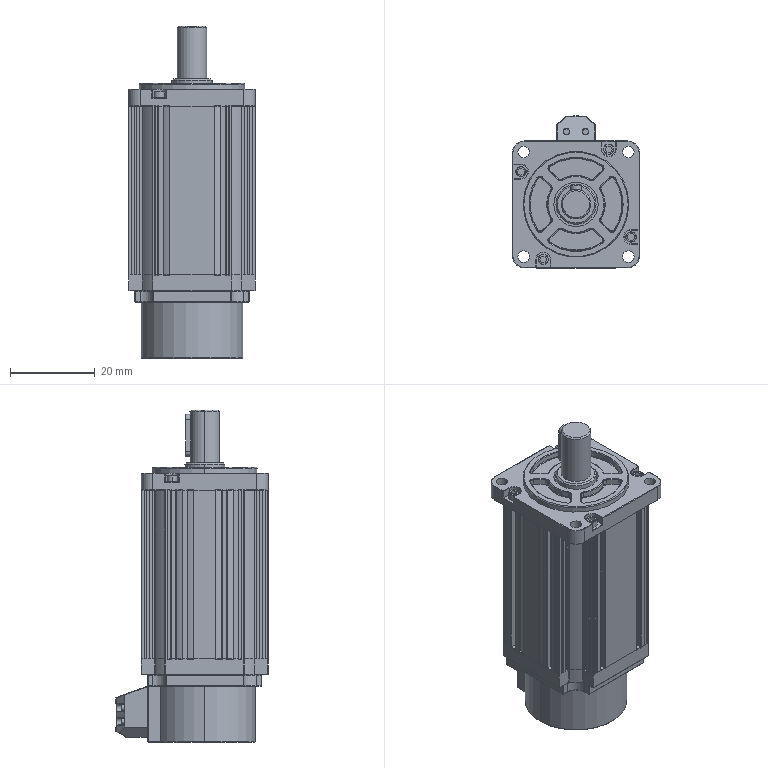Part | SolidWorks | features BaseBody 1, Scale 1 | 1 solid | 975 faces | box 30 x 36 x 78.5 mm | volume 46471 mm3 | plane 393 | cylinder 362 | torus 137 | sphere 52 | spline 24 | cone 7 | commonest cylinder face diameters 0.2 x216 1.5 x20 30 x20 0.3 x16 1.27 x8 1.8 x8